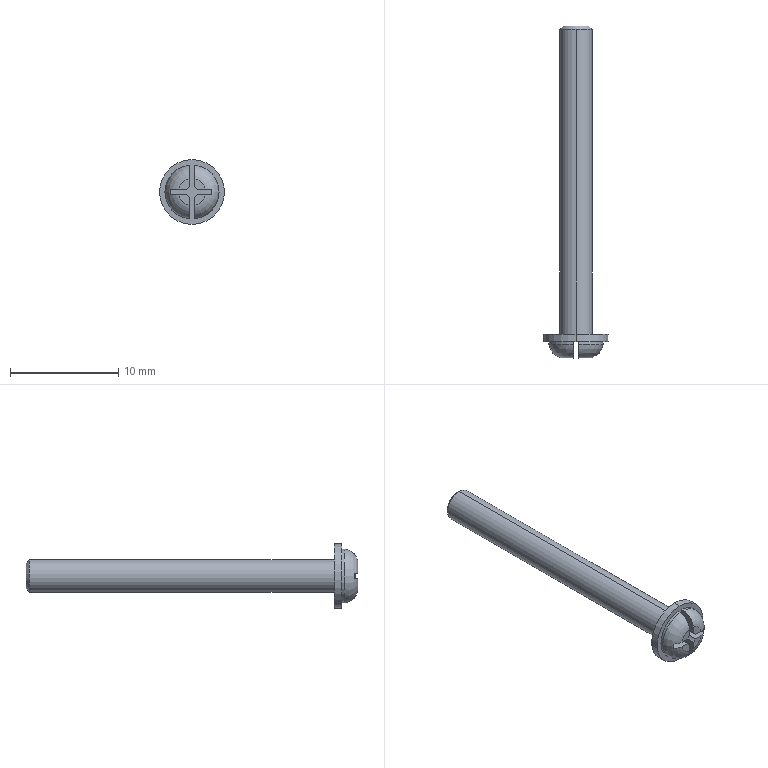Part | STEP file | 1 solid | 31 faces | box 6 x 30.7 x 6 mm | volume 238.696 mm3 | plane 17 | cylinder 10 | cone 2 | torus 2 | commonest cylinder face diameters 1.129 x4 3 x2 5 x2 6 x2
STEP:
#1=CARTESIAN_POINT('',(0.,24.019,1.2));
#2=VERTEX_POINT('',#1);
#3=CARTESIAN_POINT('',(0.,24.019,-1.2));
#4=VERTEX_POINT('',#3);
#5=CARTESIAN_POINT('',(0.,24.019,0.));
#6=DIRECTION('',(0.,1.,0.));
#7=DIRECTION('',(0.,0.,1.));
#8=AXIS2_PLACEMENT_3D('',#5,#6,#7);
#9=CIRCLE('',#8,1.2);
#10=EDGE_CURVE('',#2,#4,#9,.T.);
#11=ORIENTED_EDGE('',*,*,#10,.F.);
#12=CARTESIAN_POINT('',(0.,23.719,1.5));
#13=VERTEX_POINT('',#12);
#14=CARTESIAN_POINT('',(0.,23.719,1.5));
#15=DIRECTION('',(0.,-0.7071,0.7071));
#16=VECTOR('',#15,1000.);
#17=LINE('',#14,#16);
#18=EDGE_CURVE('',#2,#13,#17,.T.);
#19=ORIENTED_EDGE('',*,*,#18,.T.);
#20=CARTESIAN_POINT('',(0.,23.719,-1.5));
#21=VERTEX_POINT('',#20);
#22=CARTESIAN_POINT('',(0.,23.719,0.));
#23=DIRECTION('',(0.,-1.,0.));
#24=DIRECTION('',(0.,0.,1.));
#25=AXIS2_PLACEMENT_3D('',#22,#23,#24);
#26=CIRCLE('',#25,1.5);
#27=EDGE_CURVE('',#21,#13,#26,.T.);
#28=ORIENTED_EDGE('',*,*,#27,.F.);
#29=CARTESIAN_POINT('',(0.,23.719,-1.5));
#30=DIRECTION('',(0.,-0.7071,-0.7071));
#31=VECTOR('',#30,1000.);
#32=LINE('',#29,#31);
#33=EDGE_CURVE('',#4,#21,#32,.T.);
#34=ORIENTED_EDGE('',*,*,#33,.F.);
#35=EDGE_LOOP('',(#11,#19,#28,#34));
#36=FACE_OUTER_BOUND('',#35,.T.);
#37=CARTESIAN_POINT('',(0.,23.719,0.));
#38=DIRECTION('',(0.,-1.,0.));
#39=DIRECTION('',(0.,0.,-1.));
#40=AXIS2_PLACEMENT_3D('',#37,#38,#39);
#41=CONICAL_SURFACE('',#40,1.5,0.7854);
#42=ADVANCED_FACE('',(#36),#41,.T.);
#43=CARTESIAN_POINT('',(0.,-4.481,-3.));
#44=VERTEX_POINT('',#43);
#45=CARTESIAN_POINT('',(0.,-4.481,3.));
#46=VERTEX_POINT('',#45);
#47=CARTESIAN_POINT('',(0.,-4.481,0.));
#48=DIRECTION('',(0.,-1.,0.));
#49=DIRECTION('',(0.,0.,-1.));
#50=AXIS2_PLACEMENT_3D('',#47,#48,#49);
#51=CIRCLE('',#50,3.);
#52=EDGE_CURVE('',#44,#46,#51,.T.);
#53=ORIENTED_EDGE('',*,*,#52,.T.);
#54=CARTESIAN_POINT('',(0.,-5.181,3.));
#55=VERTEX_POINT('',#54);
#56=CARTESIAN_POINT('',(0.,-6.681,3.));
#57=DIRECTION('',(0.,-1.,0.));
#58=VECTOR('',#57,1000.);
#59=LINE('',#56,#58);
#60=EDGE_CURVE('',#46,#55,#59,.T.);
#61=ORIENTED_EDGE('',*,*,#60,.T.);
#62=CARTESIAN_POINT('',(0.,-5.181,-3.));
#63=VERTEX_POINT('',#62);
#64=CARTESIAN_POINT('',(0.,-5.181,0.));
#65=DIRECTION('',(0.,-1.,0.));
#66=DIRECTION('',(0.,0.,-1.));
#67=AXIS2_PLACEMENT_3D('',#64,#65,#66);
#68=CIRCLE('',#67,3.);
#69=EDGE_CURVE('',#63,#55,#68,.T.);
#70=ORIENTED_EDGE('',*,*,#69,.F.);
#71=CARTESIAN_POINT('',(0.,-6.681,-3.));
#72=DIRECTION('',(0.,-1.,0.));
#73=VECTOR('',#72,1000.);
#74=LINE('',#71,#73);
#75=EDGE_CURVE('',#44,#63,#74,.T.);
#76=ORIENTED_EDGE('',*,*,#75,.F.);
#77=EDGE_LOOP('',(#53,#61,#70,#76));
#78=FACE_OUTER_BOUND('',#77,.T.);
#79=CARTESIAN_POINT('',(0.,-6.681,0.));
#80=DIRECTION('',(0.,-1.,0.));
#81=DIRECTION('',(0.,0.,-1.));
#82=AXIS2_PLACEMENT_3D('',#79,#80,#81);
#83=CYLINDRICAL_SURFACE('',#82,3.);
#84=ADVANCED_FACE('',(#78),#83,.T.);
#85=ORIENTED_EDGE('',*,*,#27,.T.);
#86=CARTESIAN_POINT('',(0.,-4.481,1.5));
#87=VERTEX_POINT('',#86);
#88=CARTESIAN_POINT('',(0.,-6.681,1.5));
#89=DIRECTION('',(0.,-1.,0.));
#90=VECTOR('',#89,1000.);
#91=LINE('',#88,#90);
#92=EDGE_CURVE('',#13,#87,#91,.T.);
#93=ORIENTED_EDGE('',*,*,#92,.T.);
#94=CARTESIAN_POINT('',(0.,-4.481,-1.5));
#95=VERTEX_POINT('',#94);
#96=CARTESIAN_POINT('',(0.,-4.481,0.));
#97=DIRECTION('',(0.,-1.,0.));
#98=DIRECTION('',(0.,0.,-1.));
#99=AXIS2_PLACEMENT_3D('',#96,#97,#98);
#100=CIRCLE('',#99,1.5);
#101=EDGE_CURVE('',#95,#87,#100,.T.);
#102=ORIENTED_EDGE('',*,*,#101,.F.);
#103=CARTESIAN_POINT('',(0.,-6.681,-1.5));
#104=DIRECTION('',(0.,-1.,0.));
#105=VECTOR('',#104,1000.);
#106=LINE('',#103,#105);
#107=EDGE_CURVE('',#21,#95,#106,.T.);
#108=ORIENTED_EDGE('',*,*,#107,.F.);
#109=EDGE_LOOP('',(#85,#93,#102,#108));
#110=FACE_OUTER_BOUND('',#109,.T.);
#111=CARTESIAN_POINT('',(0.,-6.681,0.));
#112=DIRECTION('',(0.,-1.,0.));
#113=DIRECTION('',(0.,0.,-1.));
#114=AXIS2_PLACEMENT_3D('',#111,#112,#113);
#115=CYLINDRICAL_SURFACE('',#114,1.5);
#116=ADVANCED_FACE('',(#110),#115,.T.);
#117=CARTESIAN_POINT('',(-0.25,-5.181,2.487));
#118=VERTEX_POINT('',#117);
#119=CARTESIAN_POINT('',(-0.25,-5.431,2.487));
#120=VERTEX_POINT('',#119);
#121=CARTESIAN_POINT('',(-0.25,-6.681,2.487));
#122=DIRECTION('',(0.,-1.,0.));
#123=VECTOR('',#122,1000.);
#124=LINE('',#121,#123);
#125=EDGE_CURVE('',#118,#120,#124,.T.);
#126=ORIENTED_EDGE('',*,*,#125,.F.);
#127=CARTESIAN_POINT('',(-0.25,-5.181,-2.487));
#128=VERTEX_POINT('',#127);
#129=CARTESIAN_POINT('',(0.,-5.181,0.));
#130=DIRECTION('',(0.,-1.,0.));
#131=DIRECTION('',(0.,0.,-1.));
#132=AXIS2_PLACEMENT_3D('',#129,#130,#131);
#133=CIRCLE('',#132,2.5);
#134=EDGE_CURVE('',#118,#128,#133,.T.);
#135=ORIENTED_EDGE('',*,*,#134,.T.);
#136=CARTESIAN_POINT('',(-0.25,-5.431,-2.487));
#137=VERTEX_POINT('',#136);
#138=CARTESIAN_POINT('',(-0.25,-6.681,-2.487));
#139=DIRECTION('',(0.,1.,0.));
#140=VECTOR('',#139,1000.);
#141=LINE('',#138,#140);
#142=EDGE_CURVE('',#137,#128,#141,.T.);
#143=ORIENTED_EDGE('',*,*,#142,.F.);
#144=CARTESIAN_POINT('',(0.,-5.431,0.));
#145=DIRECTION('',(0.,-1.,0.));
#146=DIRECTION('',(0.,0.,-1.));
#147=AXIS2_PLACEMENT_3D('',#144,#145,#146);
#148=CIRCLE('',#147,2.5);
#149=EDGE_CURVE('',#120,#137,#148,.T.);
#150=ORIENTED_EDGE('',*,*,#149,.F.);
#151=EDGE_LOOP('',(#126,#135,#143,#150));
#152=FACE_OUTER_BOUND('',#151,.T.);
#153=CARTESIAN_POINT('',(0.,-6.681,0.));
#154=DIRECTION('',(0.,-1.,0.));
#155=DIRECTION('',(0.,0.,-1.));
#156=AXIS2_PLACEMENT_3D('',#153,#154,#155);
#157=CYLINDRICAL_SURFACE('',#156,2.5);
#158=ADVANCED_FACE('',(#152),#157,.T.);
#159=CARTESIAN_POINT('',(-0.25,-6.681,1.225));
#160=VERTEX_POINT('',#159);
#161=CARTESIAN_POINT('',(-0.25,-5.431,2.487));
#162=CARTESIAN_POINT('',(-0.25,-5.593,2.469));
#163=CARTESIAN_POINT('',(-0.25,-5.748,2.423));
#164=CARTESIAN_POINT('',(-0.25,-5.968,2.315));
#165=CARTESIAN_POINT('',(-0.25,-6.037,2.273));
#166=CARTESIAN_POINT('',(-0.25,-6.167,2.178));
#167=CARTESIAN_POINT('',(-0.25,-6.229,2.124));
#168=CARTESIAN_POINT('',(-0.25,-6.342,2.008));
#169=CARTESIAN_POINT('',(-0.25,-6.418,1.915));
#170=CARTESIAN_POINT('',(-0.25,-6.481,1.814));
#171=CARTESIAN_POINT('',(-0.25,-6.521,1.744));
#172=CARTESIAN_POINT('',(-0.25,-6.54,1.706));
#173=CARTESIAN_POINT('',(-0.25,-6.622,1.53));
#174=CARTESIAN_POINT('',(-0.25,-6.663,1.381));
#175=CARTESIAN_POINT('',(-0.25,-6.681,1.225));
#176=B_SPLINE_CURVE_WITH_KNOTS('',3,(#161,#162,#163,#164,#165,#166,#167,#168,#169,#170,#171,#172,#173,#174,#175),.UNSPECIFIED.,.F.,.F.,(4,2,2,2,1,2,2,4),(0.,0.25,0.375,0.5,0.625,0.6875,0.75,1.),.UNSPECIFIED.);
#177=EDGE_CURVE('',#120,#160,#176,.T.);
#178=ORIENTED_EDGE('',*,*,#177,.F.);
#179=ORIENTED_EDGE('',*,*,#149,.T.);
#180=CARTESIAN_POINT('',(-0.25,-6.681,-1.225));
#181=VERTEX_POINT('',#180);
#182=CARTESIAN_POINT('',(-0.25,-6.681,-1.225));
#183=CARTESIAN_POINT('',(-0.25,-6.671,-1.307));
#184=CARTESIAN_POINT('',(-0.25,-6.655,-1.387));
#185=CARTESIAN_POINT('',(-0.25,-6.61,-1.544));
#186=CARTESIAN_POINT('',(-0.25,-6.58,-1.622));
#187=CARTESIAN_POINT('',(-0.25,-6.476,-1.839));
#188=CARTESIAN_POINT('',(-0.25,-6.382,-1.969));
#189=CARTESIAN_POINT('',(-0.25,-6.158,-2.194));
#190=CARTESIAN_POINT('',(-0.25,-6.029,-2.285));
#191=CARTESIAN_POINT('',(-0.25,-5.74,-2.425));
#192=CARTESIAN_POINT('',(-0.25,-5.588,-2.469));
#193=CARTESIAN_POINT('',(-0.25,-5.431,-2.487));
#194=B_SPLINE_CURVE_WITH_KNOTS('',3,(#182,#183,#184,#185,#186,#187,#188,#189,#190,#191,#192,#193),.UNSPECIFIED.,.F.,.F.,(4,2,2,2,2,4),(0.,0.125,0.25,0.5,0.75,1.),.UNSPECIFIED.);
#195=EDGE_CURVE('',#181,#137,#194,.T.);
#196=ORIENTED_EDGE('',*,*,#195,.F.);
#197=CARTESIAN_POINT('',(-1.225,-6.681,-0.25));
#198=VERTEX_POINT('',#197);
#199=CARTESIAN_POINT('',(0.,-6.681,0.));
#200=DIRECTION('',(0.,-1.,0.));
#201=DIRECTION('',(0.,0.,-1.));
#202=AXIS2_PLACEMENT_3D('',#199,#200,#201);
#203=CIRCLE('',#202,1.25);
#204=EDGE_CURVE('',#198,#181,#203,.T.);
#205=ORIENTED_EDGE('',*,*,#204,.F.);
#206=CARTESIAN_POINT('',(-1.984,-6.359,-0.25));
#207=VERTEX_POINT('',#206);
#208=CARTESIAN_POINT('',(-1.984,-6.359,-0.25));
#209=CARTESIAN_POINT('',(-1.93,-6.404,-0.25));
#210=CARTESIAN_POINT('',(-1.874,-6.444,-0.25));
#211=CARTESIAN_POINT('',(-1.755,-6.516,-0.25));
#212=CARTESIAN_POINT('',(-1.691,-6.548,-0.25));
#213=CARTESIAN_POINT('',(-1.5,-6.63,-0.25));
#214=CARTESIAN_POINT('',(-1.365,-6.665,-0.25));
#215=CARTESIAN_POINT('',(-1.225,-6.681,-0.25));
#216=B_SPLINE_CURVE_WITH_KNOTS('',3,(#208,#209,#210,#211,#212,#213,#214,#215),.UNSPECIFIED.,.F.,.F.,(4,2,2,4),(0.,0.25,0.5,1.),.UNSPECIFIED.);
#217=EDGE_CURVE('',#207,#198,#216,.T.);
#218=ORIENTED_EDGE('',*,*,#217,.F.);
#219=CARTESIAN_POINT('',(-1.984,-6.359,0.25));
#220=VERTEX_POINT('',#219);
#221=CARTESIAN_POINT('',(-1.984,-6.359,0.25));
#222=CARTESIAN_POINT('',(-1.984,-6.368,0.1673));
#223=CARTESIAN_POINT('',(-1.984,-6.372,0.0837));
#224=CARTESIAN_POINT('',(-1.984,-6.372,-0.08424));
#225=CARTESIAN_POINT('',(-1.984,-6.368,-0.1675));
#226=CARTESIAN_POINT('',(-1.984,-6.359,-0.25));
#227=B_SPLINE_CURVE_WITH_KNOTS('',3,(#221,#222,#223,#224,#225,#226),.UNSPECIFIED.,.F.,.F.,(4,2,4),(0.008062,0.00831,0.008559),.UNSPECIFIED.);
#228=EDGE_CURVE('',#220,#207,#227,.T.);
#229=ORIENTED_EDGE('',*,*,#228,.F.);
#230=CARTESIAN_POINT('',(-1.225,-6.681,0.25));
#231=VERTEX_POINT('',#230);
#232=CARTESIAN_POINT('',(-1.225,-6.681,0.25));
#233=CARTESIAN_POINT('',(-1.295,-6.673,0.25));
#234=CARTESIAN_POINT('',(-1.364,-6.66,0.25));
#235=CARTESIAN_POINT('',(-1.5,-6.624,0.25));
#236=CARTESIAN_POINT('',(-1.568,-6.601,0.25));
#237=CARTESIAN_POINT('',(-1.759,-6.52,0.25));
#238=CARTESIAN_POINT('',(-1.877,-6.448,0.25));
#239=CARTESIAN_POINT('',(-1.984,-6.359,0.25));
#240=B_SPLINE_CURVE_WITH_KNOTS('',3,(#232,#233,#234,#235,#236,#237,#238,#239),.UNSPECIFIED.,.F.,.F.,(4,2,2,4),(0.,0.25,0.5,1.),.UNSPECIFIED.);
#241=EDGE_CURVE('',#231,#220,#240,.T.);
#242=ORIENTED_EDGE('',*,*,#241,.F.);
#243=CARTESIAN_POINT('',(0.,-6.681,0.));
#244=DIRECTION('',(0.,-1.,0.));
#245=DIRECTION('',(0.,0.,-1.));
#246=AXIS2_PLACEMENT_3D('',#243,#244,#245);
#247=CIRCLE('',#246,1.25);
#248=EDGE_CURVE('',#160,#231,#247,.T.);
#249=ORIENTED_EDGE('',*,*,#248,.F.);
#250=EDGE_LOOP('',(#178,#179,#196,#205,#218,#229,#242,#249));
#251=FACE_OUTER_BOUND('',#250,.T.);
#252=CARTESIAN_POINT('',(0.,-5.269,0.));
#253=DIRECTION('',(0.,-1.,0.));
#254=DIRECTION('',(0.,0.,-1.));
#255=AXIS2_PLACEMENT_3D('',#252,#253,#254);
#256=TOROIDAL_SURFACE('',#255,1.088,1.421);
#257=ADVANCED_FACE('',(#251),#256,.T.);
#258=CARTESIAN_POINT('',(0.25,-6.681,0.5061));
#259=VERTEX_POINT('',#258);
#260=CARTESIAN_POINT('',(0.25,-6.681,1.225));
#261=VERTEX_POINT('',#260);
#262=CARTESIAN_POINT('',(0.25,-6.681,2.65));
#263=DIRECTION('',(0.,0.,1.));
#264=VECTOR('',#263,1000.);
#265=LINE('',#262,#264);
#266=EDGE_CURVE('',#259,#261,#265,.T.);
#267=ORIENTED_EDGE('',*,*,#266,.F.);
#268=CARTESIAN_POINT('',(0.5061,-6.681,0.25));
#269=VERTEX_POINT('',#268);
#270=CARTESIAN_POINT('',(0.,-6.681,0.));
#271=DIRECTION('',(0.,-1.,0.));
#272=DIRECTION('',(0.,0.,-1.));
#273=AXIS2_PLACEMENT_3D('',#270,#271,#272);
#274=CIRCLE('',#273,0.5644);
#275=EDGE_CURVE('',#269,#259,#274,.T.);
#276=ORIENTED_EDGE('',*,*,#275,.F.);
#277=CARTESIAN_POINT('',(1.225,-6.681,0.25));
#278=VERTEX_POINT('',#277);
#279=CARTESIAN_POINT('',(0.,-6.681,0.25));
#280=DIRECTION('',(-1.,0.,0.));
#281=VECTOR('',#280,1000.);
#282=LINE('',#279,#281);
#283=EDGE_CURVE('',#278,#269,#282,.T.);
#284=ORIENTED_EDGE('',*,*,#283,.F.);
#285=CARTESIAN_POINT('',(0.,-6.681,0.));
#286=DIRECTION('',(0.,-1.,0.));
#287=DIRECTION('',(0.,0.,-1.));
#288=AXIS2_PLACEMENT_3D('',#285,#286,#287);
#289=CIRCLE('',#288,1.25);
#290=EDGE_CURVE('',#278,#261,#289,.T.);
#291=ORIENTED_EDGE('',*,*,#290,.T.);
#292=EDGE_LOOP('',(#267,#276,#284,#291));
#293=FACE_OUTER_BOUND('',#292,.T.);
#294=CARTESIAN_POINT('',(0.,-6.681,0.));
#295=DIRECTION('',(0.,-1.,0.));
#296=DIRECTION('',(0.,0.,-1.));
#297=AXIS2_PLACEMENT_3D('',#294,#295,#296);
#298=PLANE('',#297);
#299=ADVANCED_FACE('',(#293),#298,.T.);
#300=CARTESIAN_POINT('',(0.5061,-6.681,-0.25));
#301=VERTEX_POINT('',#300);
#302=CARTESIAN_POINT('',(1.225,-6.681,-0.25));
#303=VERTEX_POINT('',#302);
#304=CARTESIAN_POINT('',(1.793,-6.681,-0.25));
#305=DIRECTION('',(1.,0.,0.));
#306=VECTOR('',#305,1000.);
#307=LINE('',#304,#306);
#308=EDGE_CURVE('',#301,#303,#307,.T.);
#309=ORIENTED_EDGE('',*,*,#308,.F.);
#310=CARTESIAN_POINT('',(0.25,-6.681,-0.5061));
#311=VERTEX_POINT('',#310);
#312=CARTESIAN_POINT('',(0.,-6.681,0.));
#313=DIRECTION('',(0.,-1.,0.));
#314=DIRECTION('',(0.,0.,-1.));
#315=AXIS2_PLACEMENT_3D('',#312,#313,#314);
#316=CIRCLE('',#315,0.5644);
#317=EDGE_CURVE('',#311,#301,#316,.T.);
#318=ORIENTED_EDGE('',*,*,#317,.F.);
#319=CARTESIAN_POINT('',(0.25,-6.681,-1.225));
#320=VERTEX_POINT('',#319);
#321=CARTESIAN_POINT('',(0.25,-6.681,0.));
#322=DIRECTION('',(0.,0.,1.));
#323=VECTOR('',#322,1000.);
#324=LINE('',#321,#323);
#325=EDGE_CURVE('',#320,#311,#324,.T.);
#326=ORIENTED_EDGE('',*,*,#325,.F.);
#327=CARTESIAN_POINT('',(0.,-6.681,0.));
#328=DIRECTION('',(0.,-1.,0.));
#329=DIRECTION('',(0.,0.,-1.));
#330=AXIS2_PLACEMENT_3D('',#327,#328,#329);
#331=CIRCLE('',#330,1.25);
#332=EDGE_CURVE('',#320,#303,#331,.T.);
#333=ORIENTED_EDGE('',*,*,#332,.T.);
#334=EDGE_LOOP('',(#309,#318,#326,#333));
#335=FACE_OUTER_BOUND('',#334,.T.);
#336=CARTESIAN_POINT('',(0.,-6.681,0.));
#337=DIRECTION('',(0.,-1.,0.));
#338=DIRECTION('',(0.,0.,-1.));
#339=AXIS2_PLACEMENT_3D('',#336,#337,#338);
#340=PLANE('',#339);
#341=ADVANCED_FACE('',(#335),#340,.T.);
#342=CARTESIAN_POINT('',(-0.25,-6.681,-0.5061));
#343=VERTEX_POINT('',#342);
#344=CARTESIAN_POINT('',(-0.25,-6.681,-0.5061));
#345=DIRECTION('',(0.,0.,-1.));
#346=VECTOR('',#345,1000.);
#347=LINE('',#344,#346);
#348=EDGE_CURVE('',#343,#181,#347,.T.);
#349=ORIENTED_EDGE('',*,*,#348,.F.);
#350=CARTESIAN_POINT('',(-0.5061,-6.681,-0.25));
#351=VERTEX_POINT('',#350);
#352=CARTESIAN_POINT('',(0.,-6.681,0.));
#353=DIRECTION('',(0.,-1.,0.));
#354=DIRECTION('',(0.,0.,-1.));
#355=AXIS2_PLACEMENT_3D('',#352,#353,#354);
#356=CIRCLE('',#355,0.5644);
#357=EDGE_CURVE('',#351,#343,#356,.T.);
#358=ORIENTED_EDGE('',*,*,#357,.F.);
#359=CARTESIAN_POINT('',(0.,-6.681,-0.25));
#360=DIRECTION('',(1.,0.,0.));
#361=VECTOR('',#360,1000.);
#362=LINE('',#359,#361);
#363=EDGE_CURVE('',#198,#351,#362,.T.);
#364=ORIENTED_EDGE('',*,*,#363,.F.);
#365=ORIENTED_EDGE('',*,*,#204,.T.);
#366=EDGE_LOOP('',(#349,#358,#364,#365));
#367=FACE_OUTER_BOUND('',#366,.T.);
#368=CARTESIAN_POINT('',(0.,-6.681,0.));
#369=DIRECTION('',(0.,-1.,0.));
#370=DIRECTION('',(0.,0.,-1.));
#371=AXIS2_PLACEMENT_3D('',#368,#369,#370);
#372=PLANE('',#371);
#373=ADVANCED_FACE('',(#367),#372,.T.);
#374=CARTESIAN_POINT('',(0.,24.019,0.));
#375=DIRECTION('',(0.,1.,0.));
#376=DIRECTION('',(0.,0.,1.));
#377=AXIS2_PLACEMENT_3D('',#374,#375,#376);
#378=CIRCLE('',#377,1.2);
#379=EDGE_CURVE('',#4,#2,#378,.T.);
#380=ORIENTED_EDGE('',*,*,#379,.T.);
#381=ORIENTED_EDGE('',*,*,#10,.T.);
#382=EDGE_LOOP('',(#380,#381));
#383=FACE_OUTER_BOUND('',#382,.T.);
#384=CARTESIAN_POINT('',(0.,24.019,0.));
#385=DIRECTION('',(0.,1.,0.));
#386=DIRECTION('',(1.,0.,0.));
#387=AXIS2_PLACEMENT_3D('',#384,#385,#386);
#388=PLANE('',#387);
#389=ADVANCED_FACE('',(#383),#388,.T.);
#390=ORIENTED_EDGE('',*,*,#92,.F.);
#391=CARTESIAN_POINT('',(0.,23.719,0.));
#392=DIRECTION('',(0.,-1.,0.));
#393=DIRECTION('',(0.,0.,1.));
#394=AXIS2_PLACEMENT_3D('',#391,#392,#393);
#395=CIRCLE('',#394,1.5);
#396=EDGE_CURVE('',#13,#21,#395,.T.);
#397=ORIENTED_EDGE('',*,*,#396,.T.);
#398=ORIENTED_EDGE('',*,*,#107,.T.);
#399=CARTESIAN_POINT('',(0.,-4.481,0.));
#400=DIRECTION('',(0.,-1.,0.));
#401=DIRECTION('',(0.,0.,-1.));
#402=AXIS2_PLACEMENT_3D('',#399,#400,#401);
#403=CIRCLE('',#402,1.5);
#404=EDGE_CURVE('',#87,#95,#403,.T.);
#405=ORIENTED_EDGE('',*,*,#404,.F.);
#406=EDGE_LOOP('',(#390,#397,#398,#405));
#407=FACE_OUTER_BOUND('',#406,.T.);
#408=CARTESIAN_POINT('',(0.,-6.681,0.));
#409=DIRECTION('',(0.,-1.,0.));
#410=DIRECTION('',(0.,0.,-1.));
#411=AXIS2_PLACEMENT_3D('',#408,#409,#410);
#412=CYLINDRICAL_SURFACE('',#411,1.5);
#413=ADVANCED_FACE('',(#407),#412,.T.);
#414=ORIENTED_EDGE('',*,*,#52,.F.);
#415=CARTESIAN_POINT('',(0.,-4.481,0.));
#416=DIRECTION('',(0.,-1.,0.));
#417=DIRECTION('',(0.,0.,-1.));
#418=AXIS2_PLACEMENT_3D('',#415,#416,#417);
#419=CIRCLE('',#418,3.);
#420=EDGE_CURVE('',#46,#44,#419,.T.);
#421=ORIENTED_EDGE('',*,*,#420,.F.);
#422=EDGE_LOOP('',(#414,#421));
#423=FACE_OUTER_BOUND('',#422,.T.);
#424=ORIENTED_EDGE('',*,*,#101,.T.);
#425=ORIENTED_EDGE('',*,*,#404,.T.);
#426=EDGE_LOOP('',(#424,#425));
#427=FACE_BOUND('',#426,.T.);
#428=CARTESIAN_POINT('',(1.5,-4.481,0.));
#429=DIRECTION('',(0.,1.,0.));
#430=DIRECTION('',(1.,0.,0.));
#431=AXIS2_PLACEMENT_3D('',#428,#429,#430);
#432=PLANE('',#431);
#433=ADVANCED_FACE('',(#423,#427),#432,.T.);
#434=ORIENTED_EDGE('',*,*,#60,.F.);
#435=ORIENTED_EDGE('',*,*,#420,.T.);
#436=ORIENTED_EDGE('',*,*,#75,.T.);
#437=CARTESIAN_POINT('',(0.,-5.181,0.));
#438=DIRECTION('',(0.,-1.,0.));
#439=DIRECTION('',(0.,0.,-1.));
#440=AXIS2_PLACEMENT_3D('',#437,#438,#439);
#441=CIRCLE('',#440,3.);
#442=EDGE_CURVE('',#55,#63,#441,.T.);
#443=ORIENTED_EDGE('',*,*,#442,.F.);
#444=EDGE_LOOP('',(#434,#435,#436,#443));
#445=FACE_OUTER_BOUND('',#444,.T.);
#446=CARTESIAN_POINT('',(0.,-6.681,0.));
#447=DIRECTION('',(0.,-1.,0.));
#448=DIRECTION('',(0.,0.,-1.));
#449=AXIS2_PLACEMENT_3D('',#446,#447,#448);
#450=CYLINDRICAL_SURFACE('',#449,3.);
#451=ADVANCED_FACE('',(#445),#450,.T.);
#452=ORIENTED_EDGE('',*,*,#69,.T.);
#453=ORIENTED_EDGE('',*,*,#442,.T.);
#454=EDGE_LOOP('',(#452,#453));
#455=FACE_OUTER_BOUND('',#454,.T.);
#456=ORIENTED_EDGE('',*,*,#134,.F.);
#457=CARTESIAN_POINT('',(-0.25,-5.181,0.5061));
#458=VERTEX_POINT('',#457);
#459=CARTESIAN_POINT('',(-0.25,-5.181,2.65));
#460=DIRECTION('',(0.,0.,1.));
#461=VECTOR('',#460,1000.);
#462=LINE('',#459,#461);
#463=EDGE_CURVE('',#458,#118,#462,.T.);
#464=ORIENTED_EDGE('',*,*,#463,.F.);
#465=CARTESIAN_POINT('',(-0.5061,-5.181,0.25));
#466=VERTEX_POINT('',#465);
#467=CARTESIAN_POINT('',(0.,-5.181,0.));
#468=DIRECTION('',(0.,1.,0.));
#469=DIRECTION('',(0.,0.,-1.));
#470=AXIS2_PLACEMENT_3D('',#467,#468,#469);
#471=CIRCLE('',#470,0.5644);
#472=EDGE_CURVE('',#466,#458,#471,.T.);
#473=ORIENTED_EDGE('',*,*,#472,.F.);
#474=CARTESIAN_POINT('',(-1.984,-5.181,0.25));
#475=VERTEX_POINT('',#474);
#476=CARTESIAN_POINT('',(-0.5061,-5.181,0.25));
#477=DIRECTION('',(1.,0.,0.));
#478=VECTOR('',#477,1000.);
#479=LINE('',#476,#478);
#480=EDGE_CURVE('',#475,#466,#479,.T.);
#481=ORIENTED_EDGE('',*,*,#480,.F.);
#482=CARTESIAN_POINT('',(-1.984,-5.181,-0.25));
#483=VERTEX_POINT('',#482);
#484=CARTESIAN_POINT('',(-1.984,-5.181,0.25));
#485=DIRECTION('',(0.,0.,1.));
#486=VECTOR('',#485,1000.);
#487=LINE('',#484,#486);
#488=EDGE_CURVE('',#483,#475,#487,.T.);
#489=ORIENTED_EDGE('',*,*,#488,.F.);
#490=CARTESIAN_POINT('',(-0.5061,-5.181,-0.25));
#491=VERTEX_POINT('',#490);
#492=CARTESIAN_POINT('',(-0.5061,-5.181,-0.25));
#493=DIRECTION('',(-1.,0.,0.));
#494=VECTOR('',#493,1000.);
#495=LINE('',#492,#494);
#496=EDGE_CURVE('',#491,#483,#495,.T.);
#497=ORIENTED_EDGE('',*,*,#496,.F.);
#498=CARTESIAN_POINT('',(-0.25,-5.181,-0.5061));
#499=VERTEX_POINT('',#498);
#500=CARTESIAN_POINT('',(0.,-5.181,0.));
#501=DIRECTION('',(0.,1.,0.));
#502=DIRECTION('',(0.,0.,-1.));
#503=AXIS2_PLACEMENT_3D('',#500,#501,#502);
#504=CIRCLE('',#503,0.5644);
#505=EDGE_CURVE('',#499,#491,#504,.T.);
#506=ORIENTED_EDGE('',*,*,#505,.F.);
#507=CARTESIAN_POINT('',(-0.25,-5.181,-0.5061));
#508=DIRECTION('',(0.,0.,1.));
#509=VECTOR('',#508,1000.);
#510=LINE('',#507,#509);
#511=EDGE_CURVE('',#128,#499,#510,.T.);
#512=ORIENTED_EDGE('',*,*,#511,.F.);
#513=EDGE_LOOP('',(#456,#464,#473,#481,#489,#497,#506,#512));
#514=FACE_BOUND('',#513,.T.);
#515=CARTESIAN_POINT('',(0.25,-5.181,-2.487));
#516=VERTEX_POINT('',#515);
#517=CARTESIAN_POINT('',(0.25,-5.181,2.487));
#518=VERTEX_POINT('',#517);
#519=CARTESIAN_POINT('',(0.,-5.181,0.));
#520=DIRECTION('',(0.,-1.,0.));
#521=DIRECTION('',(0.,0.,-1.));
#522=AXIS2_PLACEMENT_3D('',#519,#520,#521);
#523=CIRCLE('',#522,2.5);
#524=EDGE_CURVE('',#516,#518,#523,.T.);
#525=ORIENTED_EDGE('',*,*,#524,.F.);
#526=CARTESIAN_POINT('',(0.25,-5.181,-0.5061));
#527=VERTEX_POINT('',#526);
#528=CARTESIAN_POINT('',(0.25,-5.181,-0.5061));
#529=DIRECTION('',(0.,0.,-1.));
#530=VECTOR('',#529,1000.);
#531=LINE('',#528,#530);
#532=EDGE_CURVE('',#527,#516,#531,.T.);
#533=ORIENTED_EDGE('',*,*,#532,.F.);
#534=CARTESIAN_POINT('',(0.5061,-5.181,-0.25));
#535=VERTEX_POINT('',#534);
#536=CARTESIAN_POINT('',(0.,-5.181,0.));
#537=DIRECTION('',(0.,1.,0.));
#538=DIRECTION('',(0.,0.,-1.));
#539=AXIS2_PLACEMENT_3D('',#536,#537,#538);
#540=CIRCLE('',#539,0.5644);
#541=EDGE_CURVE('',#535,#527,#540,.T.);
#542=ORIENTED_EDGE('',*,*,#541,.F.);
#543=CARTESIAN_POINT('',(1.793,-5.181,-0.25));
#544=VERTEX_POINT('',#543);
#545=CARTESIAN_POINT('',(1.793,-5.181,-0.25));
#546=DIRECTION('',(-1.,0.,0.));
#547=VECTOR('',#546,1000.);
#548=LINE('',#545,#547);
#549=EDGE_CURVE('',#544,#535,#548,.T.);
#550=ORIENTED_EDGE('',*,*,#549,.F.);
#551=CARTESIAN_POINT('',(1.793,-5.181,0.25));
#552=VERTEX_POINT('',#551);
#553=CARTESIAN_POINT('',(1.793,-5.181,-0.25));
#554=DIRECTION('',(0.,0.,-1.));
#555=VECTOR('',#554,1000.);
#556=LINE('',#553,#555);
#557=EDGE_CURVE('',#552,#544,#556,.T.);
#558=ORIENTED_EDGE('',*,*,#557,.F.);
#559=CARTESIAN_POINT('',(0.5061,-5.181,0.25));
#560=VERTEX_POINT('',#559);
#561=CARTESIAN_POINT('',(1.793,-5.181,0.25));
#562=DIRECTION('',(1.,0.,0.));
#563=VECTOR('',#562,1000.);
#564=LINE('',#561,#563);
#565=EDGE_CURVE('',#560,#552,#564,.T.);
#566=ORIENTED_EDGE('',*,*,#565,.F.);
#567=CARTESIAN_POINT('',(0.25,-5.181,0.5061));
#568=VERTEX_POINT('',#567);
#569=CARTESIAN_POINT('',(0.,-5.181,0.));
#570=DIRECTION('',(0.,1.,0.));
#571=DIRECTION('',(0.,0.,-1.));
#572=AXIS2_PLACEMENT_3D('',#569,#570,#571);
#573=CIRCLE('',#572,0.5644);
#574=EDGE_CURVE('',#568,#560,#573,.T.);
#575=ORIENTED_EDGE('',*,*,#574,.F.);
#576=CARTESIAN_POINT('',(0.25,-5.181,2.65));
#577=DIRECTION('',(0.,0.,-1.));
#578=VECTOR('',#577,1000.);
#579=LINE('',#576,#578);
#580=EDGE_CURVE('',#518,#568,#579,.T.);
#581=ORIENTED_EDGE('',*,*,#580,.F.);
#582=EDGE_LOOP('',(#525,#533,#542,#550,#558,#566,#575,#581));
#583=FACE_BOUND('',#582,.T.);
#584=CARTESIAN_POINT('',(3.,-5.181,0.));
#585=DIRECTION('',(0.,-1.,0.));
#586=DIRECTION('',(0.,0.,-1.));
#587=AXIS2_PLACEMENT_3D('',#584,#585,#586);
#588=PLANE('',#587);
#589=ADVANCED_FACE('',(#455,#514,#583),#588,.T.);
#590=CARTESIAN_POINT('',(0.25,-5.431,2.487));
#591=VERTEX_POINT('',#590);
#592=CARTESIAN_POINT('',(0.25,-6.681,2.487));
#593=DIRECTION('',(0.,1.,0.));
#594=VECTOR('',#593,1000.);
#595=LINE('',#592,#594);
#596=EDGE_CURVE('',#591,#518,#595,.T.);
#597=ORIENTED_EDGE('',*,*,#596,.F.);
#598=CARTESIAN_POINT('',(0.25,-5.431,-2.487));
#599=VERTEX_POINT('',#598);
#600=CARTESIAN_POINT('',(0.,-5.431,0.));
#601=DIRECTION('',(0.,-1.,0.));
#602=DIRECTION('',(0.,0.,-1.));
#603=AXIS2_PLACEMENT_3D('',#600,#601,#602);
#604=CIRCLE('',#603,2.5);
#605=EDGE_CURVE('',#599,#591,#604,.T.);
#606=ORIENTED_EDGE('',*,*,#605,.F.);
#607=CARTESIAN_POINT('',(0.25,-6.681,-2.487));
#608=DIRECTION('',(0.,-1.,0.));
#609=VECTOR('',#608,1000.);
#610=LINE('',#607,#609);
#611=EDGE_CURVE('',#516,#599,#610,.T.);
#612=ORIENTED_EDGE('',*,*,#611,.F.);
#613=ORIENTED_EDGE('',*,*,#524,.T.);
#614=EDGE_LOOP('',(#597,#606,#612,#613));
#615=FACE_OUTER_BOUND('',#614,.T.);
#616=CARTESIAN_POINT('',(0.,-6.681,0.));
#617=DIRECTION('',(0.,-1.,0.));
#618=DIRECTION('',(0.,0.,-1.));
#619=AXIS2_PLACEMENT_3D('',#616,#617,#618);
#620=CYLINDRICAL_SURFACE('',#619,2.5);
#621=ADVANCED_FACE('',(#615),#620,.T.);
#622=CARTESIAN_POINT('',(0.25,-6.681,1.225));
#623=CARTESIAN_POINT('',(0.25,-6.671,1.307));
#624=CARTESIAN_POINT('',(0.25,-6.655,1.387));
#625=CARTESIAN_POINT('',(0.25,-6.61,1.544));
#626=CARTESIAN_POINT('',(0.25,-6.58,1.622));
#627=CARTESIAN_POINT('',(0.25,-6.476,1.839));
#628=CARTESIAN_POINT('',(0.25,-6.382,1.969));
#629=CARTESIAN_POINT('',(0.25,-6.158,2.194));
#630=CARTESIAN_POINT('',(0.25,-6.029,2.285));
#631=CARTESIAN_POINT('',(0.25,-5.74,2.425));
#632=CARTESIAN_POINT('',(0.25,-5.588,2.469));
#633=CARTESIAN_POINT('',(0.25,-5.431,2.487));
#634=B_SPLINE_CURVE_WITH_KNOTS('',3,(#622,#623,#624,#625,#626,#627,#628,#629,#630,#631,#632,#633),.UNSPECIFIED.,.F.,.F.,(4,2,2,2,2,4),(0.,0.125,0.25,0.5,0.75,1.),.UNSPECIFIED.);
#635=EDGE_CURVE('',#261,#591,#634,.T.);
#636=ORIENTED_EDGE('',*,*,#635,.F.);
#637=ORIENTED_EDGE('',*,*,#290,.F.);
#638=CARTESIAN_POINT('',(1.793,-6.493,0.25));
#639=VERTEX_POINT('',#638);
#640=CARTESIAN_POINT('',(1.793,-6.493,0.25));
#641=CARTESIAN_POINT('',(1.618,-6.595,0.25));
#642=CARTESIAN_POINT('',(1.428,-6.658,0.25));
#643=CARTESIAN_POINT('',(1.225,-6.681,0.25));
#644=B_SPLINE_CURVE_WITH_KNOTS('',3,(#640,#641,#642,#643),.UNSPECIFIED.,.F.,.F.,(4,4),(0.,1.),.UNSPECIFIED.);
#645=EDGE_CURVE('',#639,#278,#644,.T.);
#646=ORIENTED_EDGE('',*,*,#645,.F.);
#647=CARTESIAN_POINT('',(1.793,-6.493,-0.25));
#648=VERTEX_POINT('',#647);
#649=CARTESIAN_POINT('',(1.793,-6.493,-0.25));
#650=CARTESIAN_POINT('',(1.793,-6.499,-0.1666));
#651=CARTESIAN_POINT('',(1.793,-6.503,-0.08209));
#652=CARTESIAN_POINT('',(1.793,-6.503,0.08485));
#653=CARTESIAN_POINT('',(1.793,-6.499,0.1677));
#654=CARTESIAN_POINT('',(1.793,-6.493,0.25));
#655=B_SPLINE_CURVE_WITH_KNOTS('',3,(#649,#650,#651,#652,#653,#654),.UNSPECIFIED.,.F.,.F.,(4,2,4),(0.009149,0.009395,0.009642),.UNSPECIFIED.);
#656=EDGE_CURVE('',#648,#639,#655,.T.);
#657=ORIENTED_EDGE('',*,*,#656,.F.);
#658=CARTESIAN_POINT('',(1.225,-6.681,-0.25));
#659=CARTESIAN_POINT('',(1.428,-6.658,-0.25));
#660=CARTESIAN_POINT('',(1.618,-6.595,-0.25));
#661=CARTESIAN_POINT('',(1.793,-6.493,-0.25));
#662=B_SPLINE_CURVE_WITH_KNOTS('',3,(#658,#659,#660,#661),.UNSPECIFIED.,.F.,.F.,(4,4),(0.,1.),.UNSPECIFIED.);
#663=EDGE_CURVE('',#303,#648,#662,.T.);
#664=ORIENTED_EDGE('',*,*,#663,.F.);
#665=ORIENTED_EDGE('',*,*,#332,.F.);
#666=CARTESIAN_POINT('',(0.25,-5.431,-2.487));
#667=CARTESIAN_POINT('',(0.25,-5.593,-2.469));
#668=CARTESIAN_POINT('',(0.25,-5.748,-2.423));
#669=CARTESIAN_POINT('',(0.25,-5.968,-2.315));
#670=CARTESIAN_POINT('',(0.25,-6.037,-2.273));
#671=CARTESIAN_POINT('',(0.25,-6.167,-2.178));
#672=CARTESIAN_POINT('',(0.25,-6.229,-2.124));
#673=CARTESIAN_POINT('',(0.25,-6.342,-2.008));
#674=CARTESIAN_POINT('',(0.25,-6.418,-1.915));
#675=CARTESIAN_POINT('',(0.25,-6.481,-1.814));
#676=CARTESIAN_POINT('',(0.25,-6.521,-1.744));
#677=CARTESIAN_POINT('',(0.25,-6.54,-1.706));
#678=CARTESIAN_POINT('',(0.25,-6.622,-1.53));
#679=CARTESIAN_POINT('',(0.25,-6.663,-1.381));
#680=CARTESIAN_POINT('',(0.25,-6.681,-1.225));
#681=B_SPLINE_CURVE_WITH_KNOTS('',3,(#666,#667,#668,#669,#670,#671,#672,#673,#674,#675,#676,#677,#678,#679,#680),.UNSPECIFIED.,.F.,.F.,(4,2,2,2,1,2,2,4),(0.,0.25,0.375,0.5,0.625,0.6875,0.75,1.),.UNSPECIFIED.);
#682=EDGE_CURVE('',#599,#320,#681,.T.);
#683=ORIENTED_EDGE('',*,*,#682,.F.);
#684=ORIENTED_EDGE('',*,*,#605,.T.);
#685=EDGE_LOOP('',(#636,#637,#646,#657,#664,#665,#683,#684));
#686=FACE_OUTER_BOUND('',#685,.T.);
#687=CARTESIAN_POINT('',(0.,-5.269,0.));
#688=DIRECTION('',(0.,-1.,0.));
#689=DIRECTION('',(0.,0.,-1.));
#690=AXIS2_PLACEMENT_3D('',#687,#688,#689);
#691=TOROIDAL_SURFACE('',#690,1.088,1.421);
#692=ADVANCED_FACE('',(#686),#691,.T.);
#693=CARTESIAN_POINT('',(-0.25,-6.681,0.5061));
#694=VERTEX_POINT('',#693);
#695=CARTESIAN_POINT('',(-0.25,-6.681,0.));
#696=DIRECTION('',(0.,0.,-1.));
#697=VECTOR('',#696,1000.);
#698=LINE('',#695,#697);
#699=EDGE_CURVE('',#160,#694,#698,.T.);
#700=ORIENTED_EDGE('',*,*,#699,.F.);
#701=ORIENTED_EDGE('',*,*,#248,.T.);
#702=CARTESIAN_POINT('',(-0.5061,-6.681,0.25));
#703=VERTEX_POINT('',#702);
#704=CARTESIAN_POINT('',(-0.5061,-6.681,0.25));
#705=DIRECTION('',(-1.,0.,0.));
#706=VECTOR('',#705,1000.);
#707=LINE('',#704,#706);
#708=EDGE_CURVE('',#703,#231,#707,.T.);
#709=ORIENTED_EDGE('',*,*,#708,.F.);
#710=CARTESIAN_POINT('',(0.,-6.681,0.));
#711=DIRECTION('',(0.,-1.,0.));
#712=DIRECTION('',(0.,0.,-1.));
#713=AXIS2_PLACEMENT_3D('',#710,#711,#712);
#714=CIRCLE('',#713,0.5644);
#715=EDGE_CURVE('',#694,#703,#714,.T.);
#716=ORIENTED_EDGE('',*,*,#715,.F.);
#717=EDGE_LOOP('',(#700,#701,#709,#716));
#718=FACE_OUTER_BOUND('',#717,.T.);
#719=CARTESIAN_POINT('',(0.,-6.681,0.));
#720=DIRECTION('',(0.,-1.,0.));
#721=DIRECTION('',(0.,0.,-1.));
#722=AXIS2_PLACEMENT_3D('',#719,#720,#721);
#723=PLANE('',#722);
#724=ADVANCED_FACE('',(#718),#723,.T.);
#725=ORIENTED_EDGE('',*,*,#472,.T.);
#726=CARTESIAN_POINT('',(-0.25,1.306,0.5061));
#727=DIRECTION('',(0.,-1.,0.));
#728=VECTOR('',#727,1000.);
#729=LINE('',#726,#728);
#730=EDGE_CURVE('',#458,#694,#729,.T.);
#731=ORIENTED_EDGE('',*,*,#730,.T.);
#732=ORIENTED_EDGE('',*,*,#715,.T.);
#733=CARTESIAN_POINT('',(-0.5061,1.306,0.25));
#734=DIRECTION('',(0.,-1.,0.));
#735=VECTOR('',#734,1000.);
#736=LINE('',#733,#735);
#737=EDGE_CURVE('',#466,#703,#736,.T.);
#738=ORIENTED_EDGE('',*,*,#737,.F.);
#739=EDGE_LOOP('',(#725,#731,#732,#738));
#740=FACE_OUTER_BOUND('',#739,.T.);
#741=CARTESIAN_POINT('',(0.,1.306,0.));
#742=DIRECTION('',(0.,-1.,0.));
#743=DIRECTION('',(0.,0.,-1.));
#744=AXIS2_PLACEMENT_3D('',#741,#742,#743);
#745=CYLINDRICAL_SURFACE('',#744,0.5644);
#746=ADVANCED_FACE('',(#740),#745,.F.);
#747=ORIENTED_EDGE('',*,*,#125,.T.);
#748=ORIENTED_EDGE('',*,*,#177,.T.);
#749=ORIENTED_EDGE('',*,*,#699,.T.);
#750=ORIENTED_EDGE('',*,*,#730,.F.);
#751=ORIENTED_EDGE('',*,*,#463,.T.);
#752=EDGE_LOOP('',(#747,#748,#749,#750,#751));
#753=FACE_OUTER_BOUND('',#752,.T.);
#754=CARTESIAN_POINT('',(-0.25,1.306,2.65));
#755=DIRECTION('',(-1.,0.,0.));
#756=DIRECTION('',(0.,1.,0.));
#757=AXIS2_PLACEMENT_3D('',#754,#755,#756);
#758=PLANE('',#757);
#759=ADVANCED_FACE('',(#753),#758,.F.);
#760=ORIENTED_EDGE('',*,*,#596,.T.);
#761=ORIENTED_EDGE('',*,*,#580,.T.);
#762=CARTESIAN_POINT('',(0.25,1.306,0.5061));
#763=DIRECTION('',(0.,-1.,0.));
#764=VECTOR('',#763,1000.);
#765=LINE('',#762,#764);
#766=EDGE_CURVE('',#568,#259,#765,.T.);
#767=ORIENTED_EDGE('',*,*,#766,.T.);
#768=ORIENTED_EDGE('',*,*,#266,.T.);
#769=ORIENTED_EDGE('',*,*,#635,.T.);
#770=EDGE_LOOP('',(#760,#761,#767,#768,#769));
#771=FACE_OUTER_BOUND('',#770,.T.);
#772=CARTESIAN_POINT('',(0.25,1.306,2.65));
#773=DIRECTION('',(1.,0.,0.));
#774=DIRECTION('',(0.,0.,1.));
#775=AXIS2_PLACEMENT_3D('',#772,#773,#774);
#776=PLANE('',#775);
#777=ADVANCED_FACE('',(#771),#776,.F.);
#778=ORIENTED_EDGE('',*,*,#574,.T.);
#779=CARTESIAN_POINT('',(0.5061,1.306,0.25));
#780=DIRECTION('',(0.,-1.,0.));
#781=VECTOR('',#780,1000.);
#782=LINE('',#779,#781);
#783=EDGE_CURVE('',#560,#269,#782,.T.);
#784=ORIENTED_EDGE('',*,*,#783,.T.);
#785=ORIENTED_EDGE('',*,*,#275,.T.);
#786=ORIENTED_EDGE('',*,*,#766,.F.);
#787=EDGE_LOOP('',(#778,#784,#785,#786));
#788=FACE_OUTER_BOUND('',#787,.T.);
#789=CARTESIAN_POINT('',(0.,1.306,0.));
#790=DIRECTION('',(0.,-1.,0.));
#791=DIRECTION('',(0.,0.,-1.));
#792=AXIS2_PLACEMENT_3D('',#789,#790,#791);
#793=CYLINDRICAL_SURFACE('',#792,0.5644);
#794=ADVANCED_FACE('',(#788),#793,.F.);
#795=ORIENTED_EDGE('',*,*,#645,.T.);
#796=ORIENTED_EDGE('',*,*,#283,.T.);
#797=ORIENTED_EDGE('',*,*,#783,.F.);
#798=ORIENTED_EDGE('',*,*,#565,.T.);
#799=CARTESIAN_POINT('',(1.793,1.306,0.25));
#800=DIRECTION('',(0.,-1.,0.));
#801=VECTOR('',#800,1000.);
#802=LINE('',#799,#801);
#803=EDGE_CURVE('',#552,#639,#802,.T.);
#804=ORIENTED_EDGE('',*,*,#803,.T.);
#805=EDGE_LOOP('',(#795,#796,#797,#798,#804));
#806=FACE_OUTER_BOUND('',#805,.T.);
#807=CARTESIAN_POINT('',(1.793,1.306,0.25));
#808=DIRECTION('',(0.,0.,1.));
#809=DIRECTION('',(1.,0.,0.));
#810=AXIS2_PLACEMENT_3D('',#807,#808,#809);
#811=PLANE('',#810);
#812=ADVANCED_FACE('',(#806),#811,.F.);
#813=ORIENTED_EDGE('',*,*,#656,.T.);
#814=ORIENTED_EDGE('',*,*,#803,.F.);
#815=ORIENTED_EDGE('',*,*,#557,.T.);
#816=CARTESIAN_POINT('',(1.793,1.306,-0.25));
#817=DIRECTION('',(0.,-1.,0.));
#818=VECTOR('',#817,1000.);
#819=LINE('',#816,#818);
#820=EDGE_CURVE('',#544,#648,#819,.T.);
#821=ORIENTED_EDGE('',*,*,#820,.T.);
#822=EDGE_LOOP('',(#813,#814,#815,#821));
#823=FACE_OUTER_BOUND('',#822,.T.);
#824=CARTESIAN_POINT('',(1.793,1.306,-0.25));
#825=DIRECTION('',(1.,0.,0.));
#826=DIRECTION('',(0.,1.,0.));
#827=AXIS2_PLACEMENT_3D('',#824,#825,#826);
#828=PLANE('',#827);
#829=ADVANCED_FACE('',(#823),#828,.F.);
#830=ORIENTED_EDGE('',*,*,#663,.T.);
#831=ORIENTED_EDGE('',*,*,#820,.F.);
#832=ORIENTED_EDGE('',*,*,#549,.T.);
#833=CARTESIAN_POINT('',(0.5061,1.306,-0.25));
#834=DIRECTION('',(0.,-1.,0.));
#835=VECTOR('',#834,1000.);
#836=LINE('',#833,#835);
#837=EDGE_CURVE('',#535,#301,#836,.T.);
#838=ORIENTED_EDGE('',*,*,#837,.T.);
#839=ORIENTED_EDGE('',*,*,#308,.T.);
#840=EDGE_LOOP('',(#830,#831,#832,#838,#839));
#841=FACE_OUTER_BOUND('',#840,.T.);
#842=CARTESIAN_POINT('',(1.793,1.306,-0.25));
#843=DIRECTION('',(0.,0.,-1.));
#844=DIRECTION('',(-1.,0.,0.));
#845=AXIS2_PLACEMENT_3D('',#842,#843,#844);
#846=PLANE('',#845);
#847=ADVANCED_FACE('',(#841),#846,.F.);
#848=ORIENTED_EDGE('',*,*,#541,.T.);
#849=CARTESIAN_POINT('',(0.25,1.306,-0.5061));
#850=DIRECTION('',(0.,-1.,0.));
#851=VECTOR('',#850,1000.);
#852=LINE('',#849,#851);
#853=EDGE_CURVE('',#527,#311,#852,.T.);
#854=ORIENTED_EDGE('',*,*,#853,.T.);
#855=ORIENTED_EDGE('',*,*,#317,.T.);
#856=ORIENTED_EDGE('',*,*,#837,.F.);
#857=EDGE_LOOP('',(#848,#854,#855,#856));
#858=FACE_OUTER_BOUND('',#857,.T.);
#859=CARTESIAN_POINT('',(0.,1.306,0.));
#860=DIRECTION('',(0.,-1.,0.));
#861=DIRECTION('',(0.,0.,-1.));
#862=AXIS2_PLACEMENT_3D('',#859,#860,#861);
#863=CYLINDRICAL_SURFACE('',#862,0.5644);
#864=ADVANCED_FACE('',(#858),#863,.F.);
#865=ORIENTED_EDGE('',*,*,#611,.T.);
#866=ORIENTED_EDGE('',*,*,#682,.T.);
#867=ORIENTED_EDGE('',*,*,#325,.T.);
#868=ORIENTED_EDGE('',*,*,#853,.F.);
#869=ORIENTED_EDGE('',*,*,#532,.T.);
#870=EDGE_LOOP('',(#865,#866,#867,#868,#869));
#871=FACE_OUTER_BOUND('',#870,.T.);
#872=CARTESIAN_POINT('',(0.25,1.306,-0.5061));
#873=DIRECTION('',(1.,0.,0.));
#874=DIRECTION('',(0.,0.,1.));
#875=AXIS2_PLACEMENT_3D('',#872,#873,#874);
#876=PLANE('',#875);
#877=ADVANCED_FACE('',(#871),#876,.F.);
#878=ORIENTED_EDGE('',*,*,#142,.T.);
#879=ORIENTED_EDGE('',*,*,#511,.T.);
#880=CARTESIAN_POINT('',(-0.25,1.306,-0.5061));
#881=DIRECTION('',(0.,-1.,0.));
#882=VECTOR('',#881,1000.);
#883=LINE('',#880,#882);
#884=EDGE_CURVE('',#499,#343,#883,.T.);
#885=ORIENTED_EDGE('',*,*,#884,.T.);
#886=ORIENTED_EDGE('',*,*,#348,.T.);
#887=ORIENTED_EDGE('',*,*,#195,.T.);
#888=EDGE_LOOP('',(#878,#879,#885,#886,#887));
#889=FACE_OUTER_BOUND('',#888,.T.);
#890=CARTESIAN_POINT('',(-0.25,1.306,-0.5061));
#891=DIRECTION('',(-1.,0.,0.));
#892=DIRECTION('',(0.,1.,0.));
#893=AXIS2_PLACEMENT_3D('',#890,#891,#892);
#894=PLANE('',#893);
#895=ADVANCED_FACE('',(#889),#894,.F.);
#896=ORIENTED_EDGE('',*,*,#505,.T.);
#897=CARTESIAN_POINT('',(-0.5061,1.306,-0.25));
#898=DIRECTION('',(0.,-1.,0.));
#899=VECTOR('',#898,1000.);
#900=LINE('',#897,#899);
#901=EDGE_CURVE('',#491,#351,#900,.T.);
#902=ORIENTED_EDGE('',*,*,#901,.T.);
#903=ORIENTED_EDGE('',*,*,#357,.T.);
#904=ORIENTED_EDGE('',*,*,#884,.F.);
#905=EDGE_LOOP('',(#896,#902,#903,#904));
#906=FACE_OUTER_BOUND('',#905,.T.);
#907=CARTESIAN_POINT('',(0.,1.306,0.));
#908=DIRECTION('',(0.,-1.,0.));
#909=DIRECTION('',(0.,0.,-1.));
#910=AXIS2_PLACEMENT_3D('',#907,#908,#909);
#911=CYLINDRICAL_SURFACE('',#910,0.5644);
#912=ADVANCED_FACE('',(#906),#911,.F.);
#913=ORIENTED_EDGE('',*,*,#217,.T.);
#914=ORIENTED_EDGE('',*,*,#363,.T.);
#915=ORIENTED_EDGE('',*,*,#901,.F.);
#916=ORIENTED_EDGE('',*,*,#496,.T.);
#917=CARTESIAN_POINT('',(-1.984,1.306,-0.25));
#918=DIRECTION('',(0.,-1.,0.));
#919=VECTOR('',#918,1000.);
#920=LINE('',#917,#919);
#921=EDGE_CURVE('',#483,#207,#920,.T.);
#922=ORIENTED_EDGE('',*,*,#921,.T.);
#923=EDGE_LOOP('',(#913,#914,#915,#916,#922));
#924=FACE_OUTER_BOUND('',#923,.T.);
#925=CARTESIAN_POINT('',(-0.5061,1.306,-0.25));
#926=DIRECTION('',(0.,0.,-1.));
#927=DIRECTION('',(0.,-1.,0.));
#928=AXIS2_PLACEMENT_3D('',#925,#926,#927);
#929=PLANE('',#928);
#930=ADVANCED_FACE('',(#924),#929,.F.);
#931=ORIENTED_EDGE('',*,*,#228,.T.);
#932=ORIENTED_EDGE('',*,*,#921,.F.);
#933=ORIENTED_EDGE('',*,*,#488,.T.);
#934=CARTESIAN_POINT('',(-1.984,1.306,0.25));
#935=DIRECTION('',(0.,-1.,0.));
#936=VECTOR('',#935,1000.);
#937=LINE('',#934,#936);
#938=EDGE_CURVE('',#475,#220,#937,.T.);
#939=ORIENTED_EDGE('',*,*,#938,.T.);
#940=EDGE_LOOP('',(#931,#932,#933,#939));
#941=FACE_OUTER_BOUND('',#940,.T.);
#942=CARTESIAN_POINT('',(-1.984,1.306,0.25));
#943=DIRECTION('',(-1.,0.,0.));
#944=DIRECTION('',(0.,0.,1.));
#945=AXIS2_PLACEMENT_3D('',#942,#943,#944);
#946=PLANE('',#945);
#947=ADVANCED_FACE('',(#941),#946,.F.);
#948=ORIENTED_EDGE('',*,*,#241,.T.);
#949=ORIENTED_EDGE('',*,*,#938,.F.);
#950=ORIENTED_EDGE('',*,*,#480,.T.);
#951=ORIENTED_EDGE('',*,*,#737,.T.);
#952=ORIENTED_EDGE('',*,*,#708,.T.);
#953=EDGE_LOOP('',(#948,#949,#950,#951,#952));
#954=FACE_OUTER_BOUND('',#953,.T.);
#955=CARTESIAN_POINT('',(-0.5061,1.306,0.25));
#956=DIRECTION('',(0.,0.,1.));
#957=DIRECTION('',(1.,0.,0.));
#958=AXIS2_PLACEMENT_3D('',#955,#956,#957);
#959=PLANE('',#958);
#960=ADVANCED_FACE('',(#954),#959,.F.);
#961=ORIENTED_EDGE('',*,*,#18,.F.);
#962=ORIENTED_EDGE('',*,*,#379,.F.);
#963=ORIENTED_EDGE('',*,*,#33,.T.);
#964=ORIENTED_EDGE('',*,*,#396,.F.);
#965=EDGE_LOOP('',(#961,#962,#963,#964));
#966=FACE_OUTER_BOUND('',#965,.T.);
#967=CARTESIAN_POINT('',(0.,23.719,0.));
#968=DIRECTION('',(0.,-1.,0.));
#969=DIRECTION('',(0.,0.,-1.));
#970=AXIS2_PLACEMENT_3D('',#967,#968,#969);
#971=CONICAL_SURFACE('',#970,1.5,0.7854);
#972=ADVANCED_FACE('',(#966),#971,.T.);
#973=CLOSED_SHELL('',(#42,#84,#116,#158,#257,#299,#341,#373,#389,#413,#433,#451,#589,#621,#692,#724,#746,#759,#777,#794,#812,#829,#847,#864,#877,#895,#912,#930,#947,#960,#972));
#974=MANIFOLD_SOLID_BREP('',#973);
#975=CARTESIAN_POINT('',(0.,0.,0.));
#976=DIRECTION('',(0.,0.,1.));
#977=DIRECTION('',(1.,0.,0.));
#978=AXIS2_PLACEMENT_3D('',#975,#976,#977);
#979=(LENGTH_UNIT()NAMED_UNIT(*)SI_UNIT(.MILLI.,.METRE.));
#980=UNCERTAINTY_MEASURE_WITH_UNIT(LENGTH_MEASURE(0.00001),#979,'','');
#981=(NAMED_UNIT(*)PLANE_ANGLE_UNIT()SI_UNIT($,.RADIAN.));
#982=(NAMED_UNIT(*)SI_UNIT($,.STERADIAN.)SOLID_ANGLE_UNIT());
#983=(GEOMETRIC_REPRESENTATION_CONTEXT(3)GLOBAL_UNCERTAINTY_ASSIGNED_CONTEXT((#980))GLOBAL_UNIT_ASSIGNED_CONTEXT((#979,#981,#982))REPRESENTATION_CONTEXT('',''));
#984=ADVANCED_BREP_SHAPE_REPRESENTATION('',(#974,#978),#983);